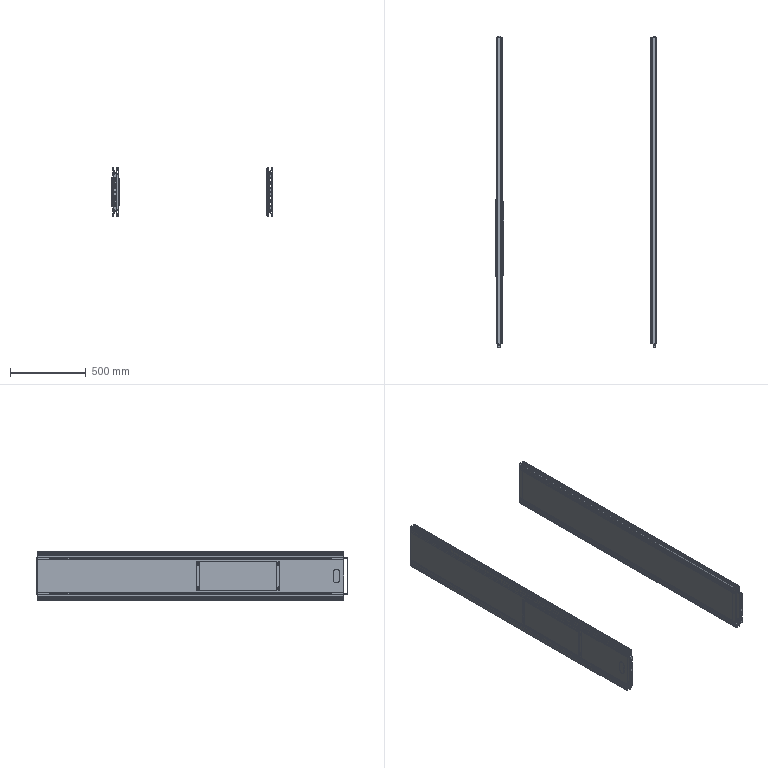Part | 53 solids | 1521 faces | box 1058 x 2051 x 320 mm | volume 12155965 mm3 | plane 922 | cylinder 599 | commonest cylinder face diameters 8.5 x80 6 x72 8 x56 6.2 x48 8.2 x48 12 x48